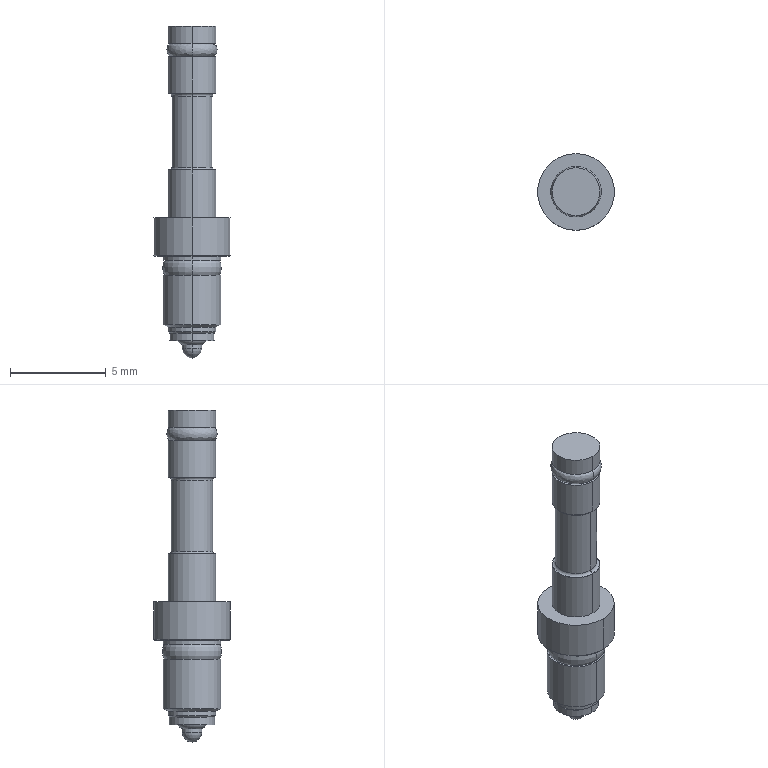Part | Creo | 1 solid | 57 faces | box 4 x 4 x 17.3 mm | volume 99.137 mm3 | cylinder 28 | plane 11 | torus 6 | cone 6 | other 4 | sphere 2 | commonest cylinder face diameters 2.5 x8 2.782 x4 3 x4 1.02 x2 2.15 x2 2.236 x2